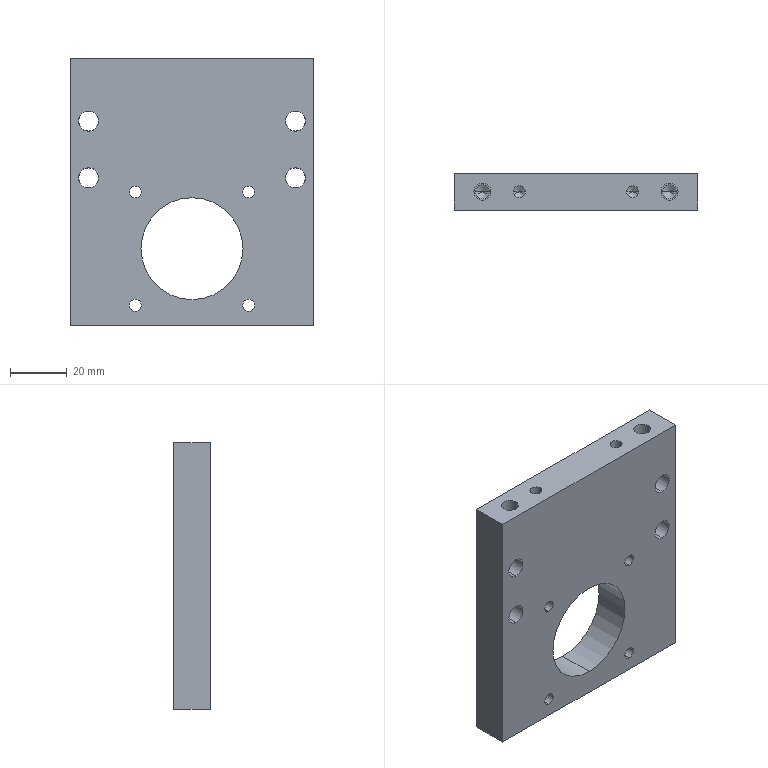Part | STEP file | OP10-119_cylinder stand (1) -R | 1 solid | 74 faces | box 86 x 13 x 94 mm | volume 86706 mm3 | cylinder 38 | cone 24 | plane 12 | commonest cylinder face diameters 4.2 x12 7 x8 11 x8 5 x4 6 x4 36 x2